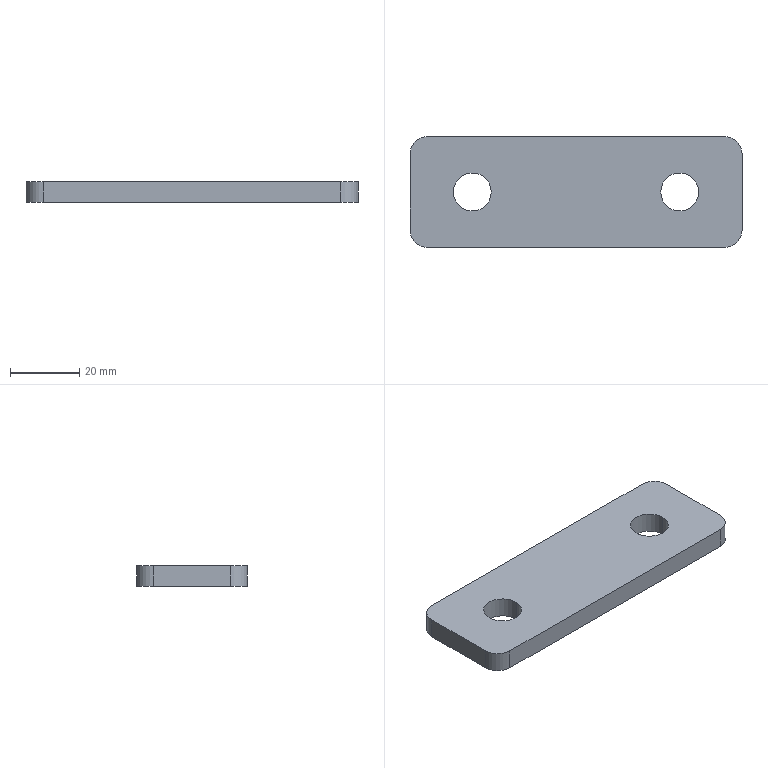Part | SolidWorks | features Extrusion 1, Fillet 1, ICE 1, LPattern 1 | 1 solid | 14 faces | box 96 x 32 x 6 mm | volume 17163 mm3 | cylinder 8 | plane 6 | commonest cylinder face diameters 10 x4 11 x4
STEP:
#1=CARTESIAN_POINT('',(72.5,-16.,0.));
#2=VERTEX_POINT('',#1);
#3=CARTESIAN_POINT('',(83.5,-16.,0.));
#4=VERTEX_POINT('',#3);
#5=CARTESIAN_POINT('',(78.,-16.,0.));
#6=DIRECTION('',(0.,0.,1.));
#7=DIRECTION('',(1.,0.,0.));
#8=AXIS2_PLACEMENT_3D('',#5,#6,#7);
#9=CIRCLE('',#8,5.5);
#10=EDGE_CURVE('',#2,#4,#9,.T.);
#11=ORIENTED_EDGE('',*,*,#10,.F.);
#12=CARTESIAN_POINT('',(72.5,-16.,6.));
#13=VERTEX_POINT('',#12);
#14=CARTESIAN_POINT('',(72.5,-16.,0.));
#15=DIRECTION('',(0.,0.,1.));
#16=VECTOR('',#15,1000.);
#17=LINE('',#14,#16);
#18=EDGE_CURVE('',#2,#13,#17,.T.);
#19=ORIENTED_EDGE('',*,*,#18,.T.);
#20=CARTESIAN_POINT('',(83.5,-16.,6.));
#21=VERTEX_POINT('',#20);
#22=CARTESIAN_POINT('',(78.,-16.,6.));
#23=DIRECTION('',(0.,0.,1.));
#24=DIRECTION('',(1.,0.,0.));
#25=AXIS2_PLACEMENT_3D('',#22,#23,#24);
#26=CIRCLE('',#25,5.5);
#27=EDGE_CURVE('',#13,#21,#26,.T.);
#28=ORIENTED_EDGE('',*,*,#27,.T.);
#29=CARTESIAN_POINT('',(83.5,-16.,0.));
#30=DIRECTION('',(0.,0.,1.));
#31=VECTOR('',#30,1000.);
#32=LINE('',#29,#31);
#33=EDGE_CURVE('',#4,#21,#32,.T.);
#34=ORIENTED_EDGE('',*,*,#33,.F.);
#35=EDGE_LOOP('',(#11,#19,#28,#34));
#36=FACE_OUTER_BOUND('',#35,.T.);
#37=CARTESIAN_POINT('',(78.,-16.,0.));
#38=DIRECTION('',(0.,0.,1.));
#39=DIRECTION('',(1.,0.,0.));
#40=AXIS2_PLACEMENT_3D('',#37,#38,#39);
#41=CYLINDRICAL_SURFACE('',#40,5.5);
#42=ADVANCED_FACE('',(#36),#41,.F.);
#43=CARTESIAN_POINT('',(12.5,-16.,0.));
#44=VERTEX_POINT('',#43);
#45=CARTESIAN_POINT('',(23.5,-16.,0.));
#46=VERTEX_POINT('',#45);
#47=CARTESIAN_POINT('',(18.,-16.,0.));
#48=DIRECTION('',(0.,0.,1.));
#49=DIRECTION('',(1.,0.,0.));
#50=AXIS2_PLACEMENT_3D('',#47,#48,#49);
#51=CIRCLE('',#50,5.5);
#52=EDGE_CURVE('',#44,#46,#51,.T.);
#53=ORIENTED_EDGE('',*,*,#52,.F.);
#54=CARTESIAN_POINT('',(12.5,-16.,6.));
#55=VERTEX_POINT('',#54);
#56=CARTESIAN_POINT('',(12.5,-16.,0.));
#57=DIRECTION('',(0.,0.,1.));
#58=VECTOR('',#57,1000.);
#59=LINE('',#56,#58);
#60=EDGE_CURVE('',#44,#55,#59,.T.);
#61=ORIENTED_EDGE('',*,*,#60,.T.);
#62=CARTESIAN_POINT('',(23.5,-16.,6.));
#63=VERTEX_POINT('',#62);
#64=CARTESIAN_POINT('',(18.,-16.,6.));
#65=DIRECTION('',(0.,0.,1.));
#66=DIRECTION('',(1.,0.,0.));
#67=AXIS2_PLACEMENT_3D('',#64,#65,#66);
#68=CIRCLE('',#67,5.5);
#69=EDGE_CURVE('',#55,#63,#68,.T.);
#70=ORIENTED_EDGE('',*,*,#69,.T.);
#71=CARTESIAN_POINT('',(23.5,-16.,0.));
#72=DIRECTION('',(0.,0.,1.));
#73=VECTOR('',#72,1000.);
#74=LINE('',#71,#73);
#75=EDGE_CURVE('',#46,#63,#74,.T.);
#76=ORIENTED_EDGE('',*,*,#75,.F.);
#77=EDGE_LOOP('',(#53,#61,#70,#76));
#78=FACE_OUTER_BOUND('',#77,.T.);
#79=CARTESIAN_POINT('',(18.,-16.,0.));
#80=DIRECTION('',(0.,0.,1.));
#81=DIRECTION('',(1.,0.,0.));
#82=AXIS2_PLACEMENT_3D('',#79,#80,#81);
#83=CYLINDRICAL_SURFACE('',#82,5.5);
#84=ADVANCED_FACE('',(#78),#83,.F.);
#85=CARTESIAN_POINT('',(0.,-5.,0.));
#86=VERTEX_POINT('',#85);
#87=CARTESIAN_POINT('',(0.,-27.,0.));
#88=VERTEX_POINT('',#87);
#89=CARTESIAN_POINT('',(0.,0.,0.));
#90=DIRECTION('',(0.,-1.,0.));
#91=VECTOR('',#90,1000.);
#92=LINE('',#89,#91);
#93=EDGE_CURVE('',#86,#88,#92,.T.);
#94=ORIENTED_EDGE('',*,*,#93,.T.);
#95=CARTESIAN_POINT('',(0.,-27.,6.));
#96=VERTEX_POINT('',#95);
#97=CARTESIAN_POINT('',(0.,-27.,6.));
#98=DIRECTION('',(0.,0.,1.));
#99=VECTOR('',#98,1000.);
#100=LINE('',#97,#99);
#101=EDGE_CURVE('',#88,#96,#100,.T.);
#102=ORIENTED_EDGE('',*,*,#101,.T.);
#103=CARTESIAN_POINT('',(0.,-5.,6.));
#104=VERTEX_POINT('',#103);
#105=CARTESIAN_POINT('',(0.,0.,6.));
#106=DIRECTION('',(0.,-1.,0.));
#107=VECTOR('',#106,1000.);
#108=LINE('',#105,#107);
#109=EDGE_CURVE('',#104,#96,#108,.T.);
#110=ORIENTED_EDGE('',*,*,#109,.F.);
#111=CARTESIAN_POINT('',(0.,-5.,6.));
#112=DIRECTION('',(0.,0.,-1.));
#113=VECTOR('',#112,1000.);
#114=LINE('',#111,#113);
#115=EDGE_CURVE('',#104,#86,#114,.T.);
#116=ORIENTED_EDGE('',*,*,#115,.T.);
#117=EDGE_LOOP('',(#94,#102,#110,#116));
#118=FACE_OUTER_BOUND('',#117,.T.);
#119=CARTESIAN_POINT('',(0.,0.,6.));
#120=DIRECTION('',(1.,0.,0.));
#121=DIRECTION('',(0.,1.,0.));
#122=AXIS2_PLACEMENT_3D('',#119,#120,#121);
#123=PLANE('',#122);
#124=ADVANCED_FACE('',(#118),#123,.F.);
#125=CARTESIAN_POINT('',(5.,-32.,0.));
#126=VERTEX_POINT('',#125);
#127=CARTESIAN_POINT('',(91.,-32.,0.));
#128=VERTEX_POINT('',#127);
#129=CARTESIAN_POINT('',(0.,-32.,0.));
#130=DIRECTION('',(1.,0.,0.));
#131=VECTOR('',#130,1000.);
#132=LINE('',#129,#131);
#133=EDGE_CURVE('',#126,#128,#132,.T.);
#134=ORIENTED_EDGE('',*,*,#133,.T.);
#135=CARTESIAN_POINT('',(91.,-32.,6.));
#136=VERTEX_POINT('',#135);
#137=CARTESIAN_POINT('',(91.,-32.,6.));
#138=DIRECTION('',(0.,0.,1.));
#139=VECTOR('',#138,1000.);
#140=LINE('',#137,#139);
#141=EDGE_CURVE('',#128,#136,#140,.T.);
#142=ORIENTED_EDGE('',*,*,#141,.T.);
#143=CARTESIAN_POINT('',(5.,-32.,6.));
#144=VERTEX_POINT('',#143);
#145=CARTESIAN_POINT('',(0.,-32.,6.));
#146=DIRECTION('',(1.,0.,0.));
#147=VECTOR('',#146,1000.);
#148=LINE('',#145,#147);
#149=EDGE_CURVE('',#144,#136,#148,.T.);
#150=ORIENTED_EDGE('',*,*,#149,.F.);
#151=CARTESIAN_POINT('',(5.,-32.,6.));
#152=DIRECTION('',(0.,0.,-1.));
#153=VECTOR('',#152,1000.);
#154=LINE('',#151,#153);
#155=EDGE_CURVE('',#144,#126,#154,.T.);
#156=ORIENTED_EDGE('',*,*,#155,.T.);
#157=EDGE_LOOP('',(#134,#142,#150,#156));
#158=FACE_OUTER_BOUND('',#157,.T.);
#159=CARTESIAN_POINT('',(0.,-32.,6.));
#160=DIRECTION('',(0.,1.,0.));
#161=DIRECTION('',(0.,0.,1.));
#162=AXIS2_PLACEMENT_3D('',#159,#160,#161);
#163=PLANE('',#162);
#164=ADVANCED_FACE('',(#158),#163,.F.);
#165=CARTESIAN_POINT('',(96.,-27.,0.));
#166=VERTEX_POINT('',#165);
#167=CARTESIAN_POINT('',(96.,-5.,0.));
#168=VERTEX_POINT('',#167);
#169=CARTESIAN_POINT('',(96.,0.,0.));
#170=DIRECTION('',(0.,1.,0.));
#171=VECTOR('',#170,1000.);
#172=LINE('',#169,#171);
#173=EDGE_CURVE('',#166,#168,#172,.T.);
#174=ORIENTED_EDGE('',*,*,#173,.T.);
#175=CARTESIAN_POINT('',(96.,-5.,6.));
#176=VERTEX_POINT('',#175);
#177=CARTESIAN_POINT('',(96.,-5.,6.));
#178=DIRECTION('',(0.,0.,1.));
#179=VECTOR('',#178,1000.);
#180=LINE('',#177,#179);
#181=EDGE_CURVE('',#168,#176,#180,.T.);
#182=ORIENTED_EDGE('',*,*,#181,.T.);
#183=CARTESIAN_POINT('',(96.,-27.,6.));
#184=VERTEX_POINT('',#183);
#185=CARTESIAN_POINT('',(96.,0.,6.));
#186=DIRECTION('',(0.,1.,0.));
#187=VECTOR('',#186,1000.);
#188=LINE('',#185,#187);
#189=EDGE_CURVE('',#184,#176,#188,.T.);
#190=ORIENTED_EDGE('',*,*,#189,.F.);
#191=CARTESIAN_POINT('',(96.,-27.,6.));
#192=DIRECTION('',(0.,0.,-1.));
#193=VECTOR('',#192,1000.);
#194=LINE('',#191,#193);
#195=EDGE_CURVE('',#184,#166,#194,.T.);
#196=ORIENTED_EDGE('',*,*,#195,.T.);
#197=EDGE_LOOP('',(#174,#182,#190,#196));
#198=FACE_OUTER_BOUND('',#197,.T.);
#199=CARTESIAN_POINT('',(96.,0.,6.));
#200=DIRECTION('',(-1.,0.,0.));
#201=DIRECTION('',(0.,0.,1.));
#202=AXIS2_PLACEMENT_3D('',#199,#200,#201);
#203=PLANE('',#202);
#204=ADVANCED_FACE('',(#198),#203,.F.);
#205=CARTESIAN_POINT('',(91.,0.,6.));
#206=VERTEX_POINT('',#205);
#207=CARTESIAN_POINT('',(5.,0.,6.));
#208=VERTEX_POINT('',#207);
#209=CARTESIAN_POINT('',(0.,0.,6.));
#210=DIRECTION('',(-1.,0.,0.));
#211=VECTOR('',#210,1000.);
#212=LINE('',#209,#211);
#213=EDGE_CURVE('',#206,#208,#212,.T.);
#214=ORIENTED_EDGE('',*,*,#213,.F.);
#215=CARTESIAN_POINT('',(91.,0.,0.));
#216=VERTEX_POINT('',#215);
#217=CARTESIAN_POINT('',(91.,0.,6.));
#218=DIRECTION('',(0.,0.,-1.));
#219=VECTOR('',#218,1000.);
#220=LINE('',#217,#219);
#221=EDGE_CURVE('',#206,#216,#220,.T.);
#222=ORIENTED_EDGE('',*,*,#221,.T.);
#223=CARTESIAN_POINT('',(5.,0.,0.));
#224=VERTEX_POINT('',#223);
#225=CARTESIAN_POINT('',(0.,0.,0.));
#226=DIRECTION('',(-1.,0.,0.));
#227=VECTOR('',#226,1000.);
#228=LINE('',#225,#227);
#229=EDGE_CURVE('',#216,#224,#228,.T.);
#230=ORIENTED_EDGE('',*,*,#229,.T.);
#231=CARTESIAN_POINT('',(5.,0.,6.));
#232=DIRECTION('',(0.,0.,1.));
#233=VECTOR('',#232,1000.);
#234=LINE('',#231,#233);
#235=EDGE_CURVE('',#224,#208,#234,.T.);
#236=ORIENTED_EDGE('',*,*,#235,.T.);
#237=EDGE_LOOP('',(#214,#222,#230,#236));
#238=FACE_OUTER_BOUND('',#237,.T.);
#239=CARTESIAN_POINT('',(0.,0.,6.));
#240=DIRECTION('',(0.,-1.,0.));
#241=DIRECTION('',(0.,0.,-1.));
#242=AXIS2_PLACEMENT_3D('',#239,#240,#241);
#243=PLANE('',#242);
#244=ADVANCED_FACE('',(#238),#243,.F.);
#245=CARTESIAN_POINT('',(78.,-16.,6.));
#246=DIRECTION('',(0.,0.,1.));
#247=DIRECTION('',(1.,0.,0.));
#248=AXIS2_PLACEMENT_3D('',#245,#246,#247);
#249=CIRCLE('',#248,5.5);
#250=EDGE_CURVE('',#21,#13,#249,.T.);
#251=ORIENTED_EDGE('',*,*,#250,.F.);
#252=ORIENTED_EDGE('',*,*,#27,.F.);
#253=EDGE_LOOP('',(#251,#252));
#254=FACE_BOUND('',#253,.T.);
#255=CARTESIAN_POINT('',(18.,-16.,6.));
#256=DIRECTION('',(0.,0.,1.));
#257=DIRECTION('',(1.,0.,0.));
#258=AXIS2_PLACEMENT_3D('',#255,#256,#257);
#259=CIRCLE('',#258,5.5);
#260=EDGE_CURVE('',#63,#55,#259,.T.);
#261=ORIENTED_EDGE('',*,*,#260,.F.);
#262=ORIENTED_EDGE('',*,*,#69,.F.);
#263=EDGE_LOOP('',(#261,#262));
#264=FACE_BOUND('',#263,.T.);
#265=ORIENTED_EDGE('',*,*,#189,.T.);
#266=CARTESIAN_POINT('',(91.,-5.,6.));
#267=DIRECTION('',(0.,0.,1.));
#268=DIRECTION('',(1.,0.,0.));
#269=AXIS2_PLACEMENT_3D('',#266,#267,#268);
#270=CIRCLE('',#269,5.);
#271=EDGE_CURVE('',#176,#206,#270,.T.);
#272=ORIENTED_EDGE('',*,*,#271,.T.);
#273=ORIENTED_EDGE('',*,*,#213,.T.);
#274=CARTESIAN_POINT('',(5.,-5.,6.));
#275=DIRECTION('',(0.,0.,1.));
#276=DIRECTION('',(1.,0.,0.));
#277=AXIS2_PLACEMENT_3D('',#274,#275,#276);
#278=CIRCLE('',#277,5.);
#279=EDGE_CURVE('',#208,#104,#278,.T.);
#280=ORIENTED_EDGE('',*,*,#279,.T.);
#281=ORIENTED_EDGE('',*,*,#109,.T.);
#282=CARTESIAN_POINT('',(5.,-27.,6.));
#283=DIRECTION('',(0.,0.,1.));
#284=DIRECTION('',(1.,0.,0.));
#285=AXIS2_PLACEMENT_3D('',#282,#283,#284);
#286=CIRCLE('',#285,5.);
#287=EDGE_CURVE('',#96,#144,#286,.T.);
#288=ORIENTED_EDGE('',*,*,#287,.T.);
#289=ORIENTED_EDGE('',*,*,#149,.T.);
#290=CARTESIAN_POINT('',(91.,-27.,6.));
#291=DIRECTION('',(0.,0.,1.));
#292=DIRECTION('',(1.,0.,0.));
#293=AXIS2_PLACEMENT_3D('',#290,#291,#292);
#294=CIRCLE('',#293,5.);
#295=EDGE_CURVE('',#136,#184,#294,.T.);
#296=ORIENTED_EDGE('',*,*,#295,.T.);
#297=EDGE_LOOP('',(#265,#272,#273,#280,#281,#288,#289,#296));
#298=FACE_OUTER_BOUND('',#297,.T.);
#299=CARTESIAN_POINT('',(0.,0.,6.));
#300=DIRECTION('',(0.,0.,1.));
#301=DIRECTION('',(1.,0.,0.));
#302=AXIS2_PLACEMENT_3D('',#299,#300,#301);
#303=PLANE('',#302);
#304=ADVANCED_FACE('',(#254,#264,#298),#303,.T.);
#305=CARTESIAN_POINT('',(78.,-16.,0.));
#306=DIRECTION('',(0.,0.,1.));
#307=DIRECTION('',(1.,0.,0.));
#308=AXIS2_PLACEMENT_3D('',#305,#306,#307);
#309=CIRCLE('',#308,5.5);
#310=EDGE_CURVE('',#4,#2,#309,.T.);
#311=ORIENTED_EDGE('',*,*,#310,.T.);
#312=ORIENTED_EDGE('',*,*,#10,.T.);
#313=EDGE_LOOP('',(#311,#312));
#314=FACE_BOUND('',#313,.T.);
#315=CARTESIAN_POINT('',(18.,-16.,0.));
#316=DIRECTION('',(0.,0.,1.));
#317=DIRECTION('',(1.,0.,0.));
#318=AXIS2_PLACEMENT_3D('',#315,#316,#317);
#319=CIRCLE('',#318,5.5);
#320=EDGE_CURVE('',#46,#44,#319,.T.);
#321=ORIENTED_EDGE('',*,*,#320,.T.);
#322=ORIENTED_EDGE('',*,*,#52,.T.);
#323=EDGE_LOOP('',(#321,#322));
#324=FACE_BOUND('',#323,.T.);
#325=ORIENTED_EDGE('',*,*,#229,.F.);
#326=CARTESIAN_POINT('',(91.,-5.,0.));
#327=DIRECTION('',(0.,0.,-1.));
#328=DIRECTION('',(1.,0.,0.));
#329=AXIS2_PLACEMENT_3D('',#326,#327,#328);
#330=CIRCLE('',#329,5.);
#331=EDGE_CURVE('',#216,#168,#330,.T.);
#332=ORIENTED_EDGE('',*,*,#331,.T.);
#333=ORIENTED_EDGE('',*,*,#173,.F.);
#334=CARTESIAN_POINT('',(91.,-27.,0.));
#335=DIRECTION('',(0.,0.,-1.));
#336=DIRECTION('',(1.,0.,0.));
#337=AXIS2_PLACEMENT_3D('',#334,#335,#336);
#338=CIRCLE('',#337,5.);
#339=EDGE_CURVE('',#166,#128,#338,.T.);
#340=ORIENTED_EDGE('',*,*,#339,.T.);
#341=ORIENTED_EDGE('',*,*,#133,.F.);
#342=CARTESIAN_POINT('',(5.,-27.,0.));
#343=DIRECTION('',(0.,0.,-1.));
#344=DIRECTION('',(1.,0.,0.));
#345=AXIS2_PLACEMENT_3D('',#342,#343,#344);
#346=CIRCLE('',#345,5.);
#347=EDGE_CURVE('',#126,#88,#346,.T.);
#348=ORIENTED_EDGE('',*,*,#347,.T.);
#349=ORIENTED_EDGE('',*,*,#93,.F.);
#350=CARTESIAN_POINT('',(5.,-5.,0.));
#351=DIRECTION('',(0.,0.,-1.));
#352=DIRECTION('',(1.,0.,0.));
#353=AXIS2_PLACEMENT_3D('',#350,#351,#352);
#354=CIRCLE('',#353,5.);
#355=EDGE_CURVE('',#86,#224,#354,.T.);
#356=ORIENTED_EDGE('',*,*,#355,.T.);
#357=EDGE_LOOP('',(#325,#332,#333,#340,#341,#348,#349,#356));
#358=FACE_OUTER_BOUND('',#357,.T.);
#359=CARTESIAN_POINT('',(0.,0.,0.));
#360=DIRECTION('',(0.,0.,1.));
#361=DIRECTION('',(1.,0.,0.));
#362=AXIS2_PLACEMENT_3D('',#359,#360,#361);
#363=PLANE('',#362);
#364=ADVANCED_FACE('',(#314,#324,#358),#363,.F.);
#365=ORIENTED_EDGE('',*,*,#271,.F.);
#366=ORIENTED_EDGE('',*,*,#181,.F.);
#367=ORIENTED_EDGE('',*,*,#331,.F.);
#368=ORIENTED_EDGE('',*,*,#221,.F.);
#369=EDGE_LOOP('',(#365,#366,#367,#368));
#370=FACE_OUTER_BOUND('',#369,.T.);
#371=CARTESIAN_POINT('',(91.,-5.,6.));
#372=DIRECTION('',(0.,0.,-1.));
#373=DIRECTION('',(-1.,0.,0.));
#374=AXIS2_PLACEMENT_3D('',#371,#372,#373);
#375=CYLINDRICAL_SURFACE('',#374,5.);
#376=ADVANCED_FACE('',(#370),#375,.T.);
#377=ORIENTED_EDGE('',*,*,#295,.F.);
#378=ORIENTED_EDGE('',*,*,#141,.F.);
#379=ORIENTED_EDGE('',*,*,#339,.F.);
#380=ORIENTED_EDGE('',*,*,#195,.F.);
#381=EDGE_LOOP('',(#377,#378,#379,#380));
#382=FACE_OUTER_BOUND('',#381,.T.);
#383=CARTESIAN_POINT('',(91.,-27.,6.));
#384=DIRECTION('',(0.,0.,-1.));
#385=DIRECTION('',(-1.,0.,0.));
#386=AXIS2_PLACEMENT_3D('',#383,#384,#385);
#387=CYLINDRICAL_SURFACE('',#386,5.);
#388=ADVANCED_FACE('',(#382),#387,.T.);
#389=ORIENTED_EDGE('',*,*,#287,.F.);
#390=ORIENTED_EDGE('',*,*,#101,.F.);
#391=ORIENTED_EDGE('',*,*,#347,.F.);
#392=ORIENTED_EDGE('',*,*,#155,.F.);
#393=EDGE_LOOP('',(#389,#390,#391,#392));
#394=FACE_OUTER_BOUND('',#393,.T.);
#395=CARTESIAN_POINT('',(5.,-27.,6.));
#396=DIRECTION('',(0.,0.,-1.));
#397=DIRECTION('',(-1.,0.,0.));
#398=AXIS2_PLACEMENT_3D('',#395,#396,#397);
#399=CYLINDRICAL_SURFACE('',#398,5.);
#400=ADVANCED_FACE('',(#394),#399,.T.);
#401=ORIENTED_EDGE('',*,*,#279,.F.);
#402=ORIENTED_EDGE('',*,*,#235,.F.);
#403=ORIENTED_EDGE('',*,*,#355,.F.);
#404=ORIENTED_EDGE('',*,*,#115,.F.);
#405=EDGE_LOOP('',(#401,#402,#403,#404));
#406=FACE_OUTER_BOUND('',#405,.T.);
#407=CARTESIAN_POINT('',(5.,-5.,6.));
#408=DIRECTION('',(0.,0.,-1.));
#409=DIRECTION('',(-1.,0.,0.));
#410=AXIS2_PLACEMENT_3D('',#407,#408,#409);
#411=CYLINDRICAL_SURFACE('',#410,5.);
#412=ADVANCED_FACE('',(#406),#411,.T.);
#413=ORIENTED_EDGE('',*,*,#60,.F.);
#414=ORIENTED_EDGE('',*,*,#320,.F.);
#415=ORIENTED_EDGE('',*,*,#75,.T.);
#416=ORIENTED_EDGE('',*,*,#260,.T.);
#417=EDGE_LOOP('',(#413,#414,#415,#416));
#418=FACE_OUTER_BOUND('',#417,.T.);
#419=CARTESIAN_POINT('',(18.,-16.,0.));
#420=DIRECTION('',(0.,0.,1.));
#421=DIRECTION('',(1.,0.,0.));
#422=AXIS2_PLACEMENT_3D('',#419,#420,#421);
#423=CYLINDRICAL_SURFACE('',#422,5.5);
#424=ADVANCED_FACE('',(#418),#423,.F.);
#425=ORIENTED_EDGE('',*,*,#18,.F.);
#426=ORIENTED_EDGE('',*,*,#310,.F.);
#427=ORIENTED_EDGE('',*,*,#33,.T.);
#428=ORIENTED_EDGE('',*,*,#250,.T.);
#429=EDGE_LOOP('',(#425,#426,#427,#428));
#430=FACE_OUTER_BOUND('',#429,.T.);
#431=CARTESIAN_POINT('',(78.,-16.,0.));
#432=DIRECTION('',(0.,0.,1.));
#433=DIRECTION('',(1.,0.,0.));
#434=AXIS2_PLACEMENT_3D('',#431,#432,#433);
#435=CYLINDRICAL_SURFACE('',#434,5.5);
#436=ADVANCED_FACE('',(#430),#435,.F.);
#437=CLOSED_SHELL('',(#42,#84,#124,#164,#204,#244,#304,#364,#376,#388,#400,#412,#424,#436));
#438=MANIFOLD_SOLID_BREP('',#437);
#439=CARTESIAN_POINT('',(0.,0.,0.));
#440=DIRECTION('',(0.,0.,1.));
#441=DIRECTION('',(1.,0.,0.));
#442=AXIS2_PLACEMENT_3D('',#439,#440,#441);
#443=(LENGTH_UNIT()NAMED_UNIT(*)SI_UNIT(.MILLI.,.METRE.));
#444=UNCERTAINTY_MEASURE_WITH_UNIT(LENGTH_MEASURE(0.00001),#443,'','');
#445=(NAMED_UNIT(*)PLANE_ANGLE_UNIT()SI_UNIT($,.RADIAN.));
#446=(NAMED_UNIT(*)SI_UNIT($,.STERADIAN.)SOLID_ANGLE_UNIT());
#447=(GEOMETRIC_REPRESENTATION_CONTEXT(3)GLOBAL_UNCERTAINTY_ASSIGNED_CONTEXT((#444))GLOBAL_UNIT_ASSIGNED_CONTEXT((#443,#445,#446))REPRESENTATION_CONTEXT('',''));
#448=ADVANCED_BREP_SHAPE_REPRESENTATION('',(#438,#442),#447);